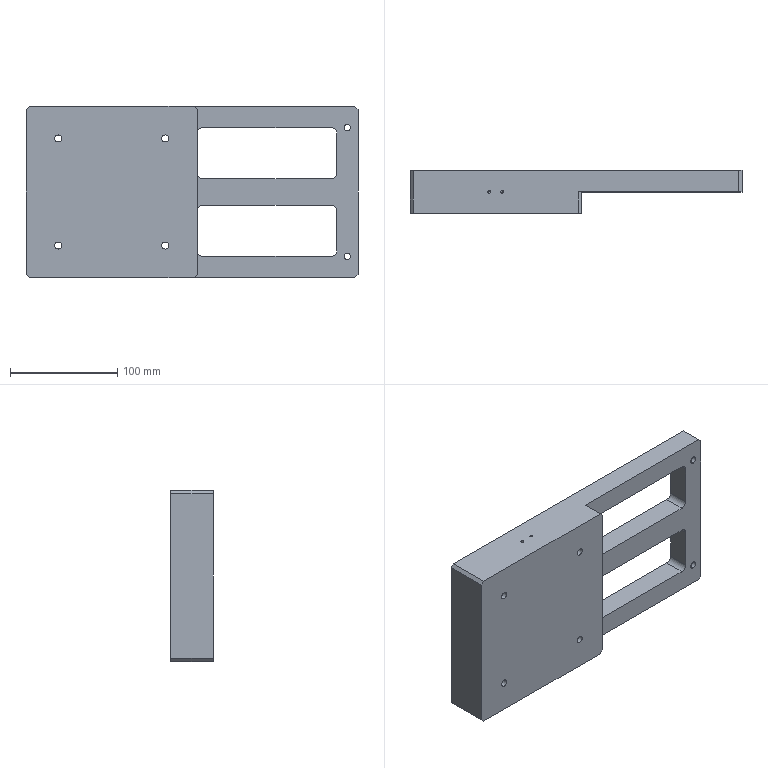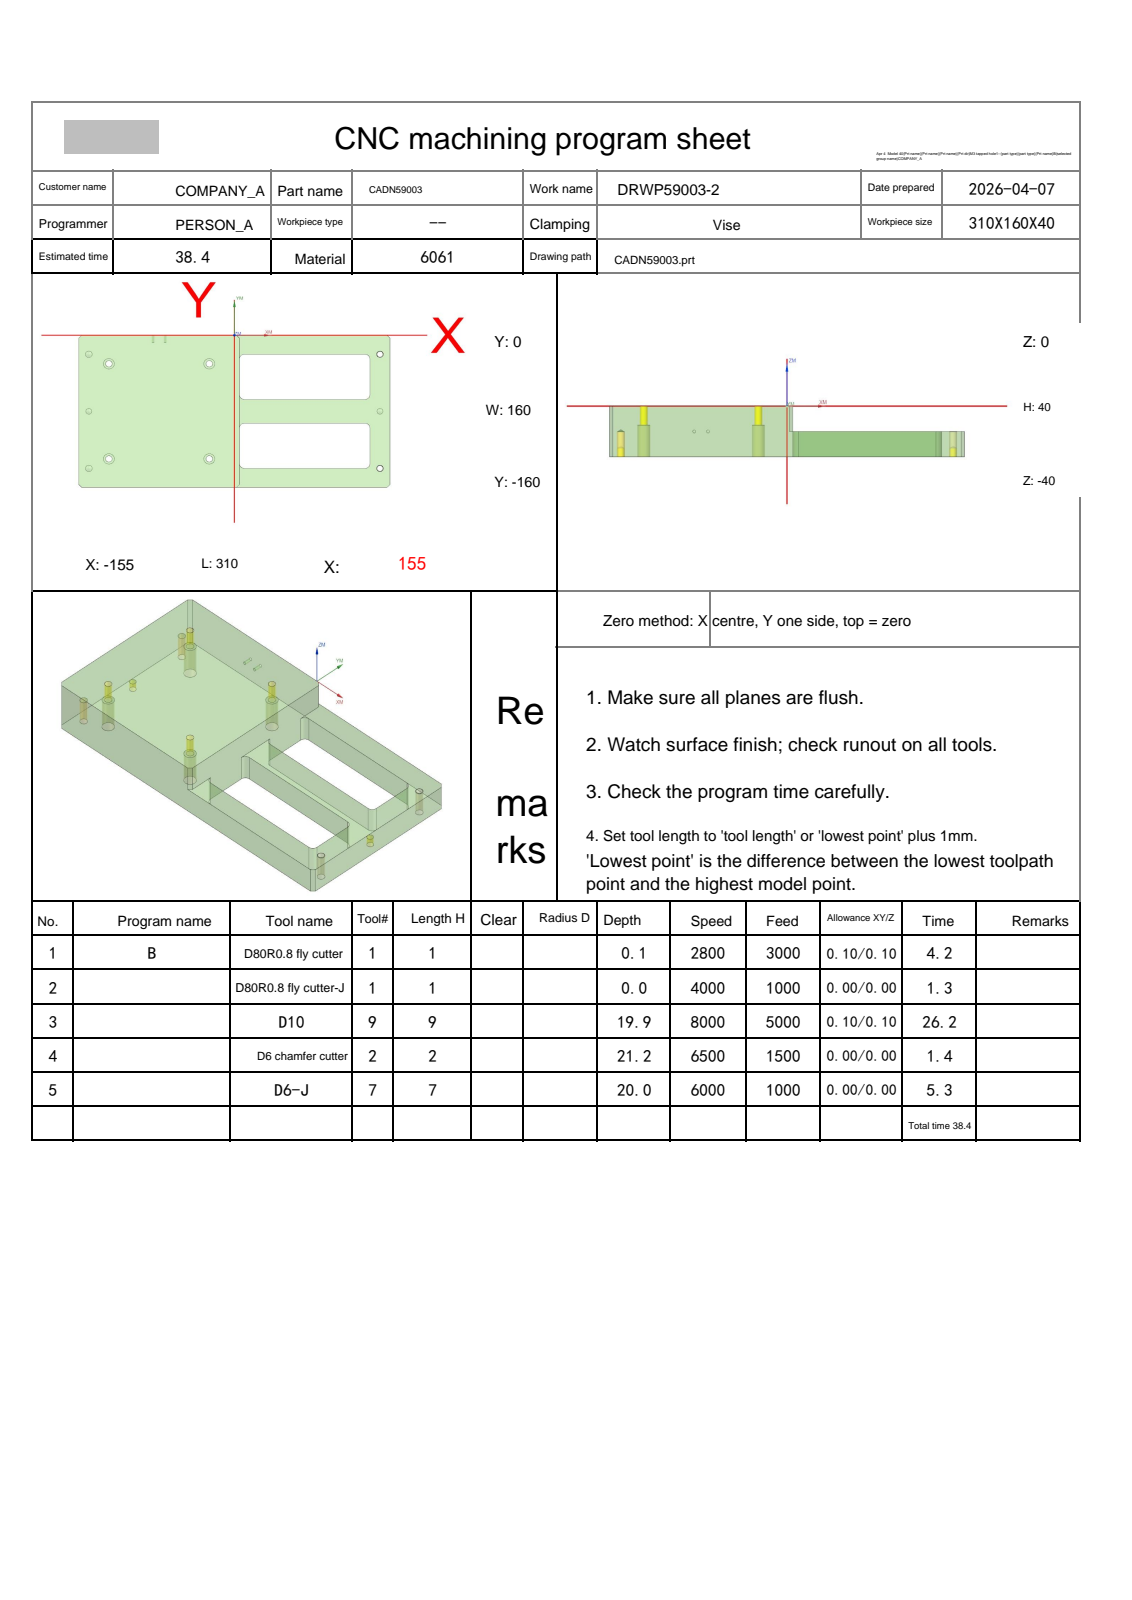NC program | NX | posted by the shop | part box 310 x 40 x 160 mm
Lines 5366 to 6465 of 6465:
N4 T02 M06
(D6 chamfer cutter  D=6. R=0. H=02 ce=0.00 di=0.00)
G00 G90 G54 X-74.614 Y-161.227 M03 S6500
G43 H02 Z20.
M08
Z.172
G01 Z-1.2 F1500.
G03 X-74.9 Y-161.027 I-1.286 J-1.532
G01 X-74.946 Y-160.997
X-75. Y-161.
X-152.
X-152.259 Y-160.966
X-152.5 Y-160.866
X-152.707 Y-160.707
X-155.707 Y-157.707
X-155.866 Y-157.5
X-155.966 Y-157.259
X-156. Y-157.
Y-3.
X-155.966 Y-2.741
X-155.866 Y-2.5
X-155.707 Y-2.293
X-152.707 Y.707
X-152.5 Y.866
X-152.259 Y.966
X-152. Y1.
X2.
X2.259 Y.966
X2.5 Y.866
X2.707 Y.707
X5.707 Y-2.293
X5.866 Y-2.5
X5.966 Y-2.741
X6. Y-3.
Y-157.
X5.966 Y-157.259
X5.866 Y-157.5
X5.707 Y-157.707
X2.707 Y-160.707
X2.5 Y-160.866
X2.259 Y-160.966
X2. Y-161.
X-75.
X-75.054 Y-160.997
X-75.1 Y-161.027
G03 X-75.386 Y-161.227 I1. J-1.732
G01 Z.172
G00 Z10.
X-24.596 Y-127.892
Z.253
G01 Z-1.2
G03 X-24.898 Y-127.718 I-1.147 J-1.638
G01 X-24.946 Y-127.692
X-25. Y-127.7
G03 X-27.3 Y-130. I0.0 J-2.3
X-25. Y-132.3 I2.3 J0.0
X-22.7 Y-130. I0.0 J2.3
X-25. Y-127.7 I-2.3 J0.0
G01 X-25.054 Y-127.692
X-25.102 Y-127.718
G03 X-25.404 Y-127.892 I.845 J-1.813
G01 Z.253
G00 Z10.
X-124.596
Z.253
G01 Z-1.2
G03 X-124.898 Y-127.718 I-1.147 J-1.638
G01 X-124.946 Y-127.692
X-125. Y-127.7
G03 X-127.3 Y-130. I0.0 J-2.3
X-125. Y-132.3 I2.3 J0.0
X-122.7 Y-130. I0.0 J2.3
X-125. Y-127.7 I-2.3 J0.0
G01 X-125.054 Y-127.692
X-125.102 Y-127.718
G03 X-125.404 Y-127.892 I.845 J-1.813
G01 Z.253
G00 Z10.
X-124.596 Y-27.892
Z.253
G01 Z-1.2
G03 X-124.898 Y-27.718 I-1.147 J-1.638
G01 X-124.946 Y-27.692
X-125. Y-27.7
G03 X-127.3 Y-30. I0.0 J-2.3
X-125. Y-32.3 I2.3 J0.0
X-122.7 Y-30. I0.0 J2.3
X-125. Y-27.7 I-2.3 J0.0
G01 X-125.054 Y-27.692
X-125.102 Y-27.718
G03 X-125.404 Y-27.892 I.845 J-1.813
G01 Z.253
G00 Z10.
X-24.596
Z.253
G01 Z-1.2
G03 X-24.898 Y-27.718 I-1.147 J-1.638
G01 X-24.946 Y-27.692
X-25. Y-27.7
G03 X-27.3 Y-30. I0.0 J-2.3
X-25. Y-32.3 I2.3 J0.0
X-22.7 Y-30. I0.0 J2.3
X-25. Y-27.7 I-2.3 J0.0
G01 X-25.054 Y-27.692
X-25.102 Y-27.718
G03 X-25.404 Y-27.892 I.845 J-1.813
G01 Z.253
G00 Z10.
X8.195 Y-65.959
Z-1.796
G01 Z-21.199
X8.217 Y-66.027
X8.262 Y-66.081
X8.269 Y-66.105
X8.293 Y-66.109
X8.469 Y-66.196
X8.965 Y-66.364
X9.478 Y-66.466
X10. Y-66.5
X130.
G03 X134. Y-62.5 I0.0 J4.
G01 Y-25.
G03 X130. Y-21. I-4. J0.0
G01 X10.
X9.478 Y-21.034
X8.965 Y-21.136
X8.469 Y-21.304
X8.293 Y-21.391
X8.271 Y-21.405
X8.249 Y-21.427
X8.206 Y-21.523
Z-1.807
G00 Z10.
X8.195 Y-138.459
Z-1.796
G01 Z-21.199
X8.217 Y-138.527
X8.262 Y-138.581
X8.269 Y-138.605
X8.293 Y-138.609
X8.469 Y-138.696
X8.965 Y-138.864
X9.478 Y-138.966
X10. Y-139.
X130.
G03 X134. Y-135. I0.0 J4.
G01 Y-97.5
G03 X130. Y-93.5 I-4. J0.0
G01 X10.
X9.478 Y-93.534
X8.965 Y-93.636
X8.469 Y-93.804
X8.293 Y-93.891
X8.271 Y-93.905
X8.249 Y-93.927
X8.206 Y-94.023
Z-1.807
G00 Z10.
X5.356 Y1.159
Z-1.793
G01 Z-21.199
G03 X5.555 Y1.019 I.9 J1.072
G01 X5.587 Y.995
X5.625 Y1.
X152.
X152.259 Y.966
X152.5 Y.866
X152.707 Y.707
X155.707 Y-2.293
X155.866 Y-2.5
X155.966 Y-2.741
X156. Y-3.
Y-157.
X155.966 Y-157.259
X155.866 Y-157.5
X155.707 Y-157.707
X152.707 Y-160.707
X152.5 Y-160.866
X152.259 Y-160.966
X152. Y-161.
X5.625
X5.587 Y-160.995
X5.555 Y-161.019
G03 X5.356 Y-161.159 I.7 J-1.212
G01 Z-1.793
G00 Z10.
X145.404 Y-18.208
Z-19.74
G01 Z-21.199
G03 X145.102 Y-18.034 I-1.147 J-1.638
G01 X145.054 Y-18.009
X145. Y-18.016
G03 X143.016 Y-20. I0.0 J-1.984
X145. Y-21.984 I1.984 J0.0
X146.984 Y-20. I0.0 J1.984
X145.345 Y-18.046 I-1.984 J0.0
G01 X145. Y-18.016
X144.946 Y-18.009
X144.898 Y-18.034
G03 X144.596 Y-18.208 I.845 J-1.813
G01 Z-19.74
G00 Z10.
X145.404 Y-138.208
Z-19.74
G01 Z-21.199
G03 X145.102 Y-138.034 I-1.147 J-1.638
G01 X145.054 Y-138.009
X145. Y-138.016
G03 X143.016 Y-140. I0.0 J-1.984
X145. Y-141.984 I1.984 J0.0
X146.984 Y-140. I0.0 J1.984
X145.345 Y-138.046 I-1.984 J0.0
G01 X145. Y-138.016
X144.946 Y-138.009
X144.898 Y-138.034
G03 X144.596 Y-138.208 I.845 J-1.813
G01 Z-19.74
G00 Z20.
G91 G28 Z0.0
M05
M09
G91 G28 Z0.0
M01
N5 T07 M06
(D6-J  D=6. R=0. H=07 ce=0.40 di=0.00)
G00 G90 G54 X158.917 Y-158.649 M03 S6000
G43 H07 Z14.5
M08
Z-18.5
G01 Z-20. F1000.
X156.6
G02 X155.4 Y-157.449 I0.0 J1.2
G01 Y-139.099
G03 X153.626 Y-116.329 I-147. J0.0
G01 X153.611 Y-116.25
X153.626 Y-116.171
G03 X155.4 Y-93.401 I-145.226 J22.77
G01 Y-66.599
G03 X153.626 Y-43.829 I-147. J0.0
G01 X153.611 Y-43.75
X153.626 Y-43.671
G03 X155.4 Y-20.901 I-145.226 J22.77
G01 Y-2.8
G03 X155.224 Y-2.376 I-.6 J0.0
G01 X152.802 Y.046
X152.633 Y.117
G03 X152.393 Y-.123 I0.0 J-.24
G01 Y-.126
G02 X152.4 Y-1.584 I-143.993 J-1.466
G01 Y-20.901
G02 X150.589 Y-43.669 I-144. J0.0
G01 X150.573 Y-43.75
X150.589 Y-43.831
G02 X152.4 Y-66.599 I-142.189 J-22.768
G01 Y-93.401
G02 X150.589 Y-116.169 I-144. J0.0
G01 X150.573 Y-116.25
X150.589 Y-116.331
G02 X152.4 Y-139.099 I-142.189 J-22.768
G01 Y-158.408
G02 X152.39 Y-160.066 I-144. J0.0
X151.851 Y-160.6 I-.54 J.006
G01 X149.93
G02 X149.39 Y-160.06 I0.0 J.54
G01 Y-160.054
G03 X149.4 Y-158.408 I-140.99 J1.646
G01 Y-139.099
G03 X147.55 Y-116.333 I-141. J0.0
G01 X147.534 Y-116.25
X147.55 Y-116.167
G03 X149.4 Y-93.401 I-139.15 J22.766
G01 Y-66.599
G03 X147.55 Y-43.833 I-141. J0.0
G01 X147.534 Y-43.75
X147.55 Y-43.667
G03 X149.4 Y-20.901 I-139.15 J22.766
G01 Y-1.584
G03 X149.391 Y.007 I-141. J-.008
X148.791 Y.6 I-.6 J-.007
G01 X146.93
G03 X146.39 Y.06 I0.0 J-.54
G01 Y.054
G02 X146.4 Y-1.584 I-137.99 J-1.646
G01 Y-20.901
G02 X144.51 Y-43.664 I-138. J0.0
G01 X144.494 Y-43.75
X144.51 Y-43.836
G02 X146.4 Y-66.599 I-136.11 J-22.763
G01 Y-93.401
G02 X144.51 Y-116.164 I-138. J0.0
G01 X144.494 Y-116.25
X144.51 Y-116.336
G02 X146.4 Y-139.099 I-136.11 J-22.763
G01 Y-158.408
G02 X146.391 Y-160.007 I-138. J0.0
X145.791 Y-160.6 I-.6 J.007
G01 X143.93
G02 X143.39 Y-160.06 I0.0 J.54
G01 Y-160.054
G03 X143.4 Y-158.408 I-134.99 J1.645
G01 Y-139.099
G03 X141.467 Y-116.338 I-135. J0.0
G01 X141.451 Y-116.25
X141.467 Y-116.162
G03 X143.4 Y-93.401 I-133.067 J22.761
G01 Y-66.599
G03 X141.467 Y-43.838 I-135. J0.0
G01 X141.451 Y-43.75
X141.467 Y-43.662
G03 X143.4 Y-20.901 I-133.067 J22.761
G01 Y-1.584
G03 X143.391 Y.007 I-135. J-.008
X142.791 Y.6 I-.6 J-.007
G01 X140.929
G03 X140.39 Y.06 I0.0 J-.54
G01 Y.054
G02 X140.4 Y-1.584 I-131.99 J-1.645
G01 Y-20.901
G02 X138.423 Y-43.659 I-132. J0.0
G01 X138.406 Y-43.75
X138.423 Y-43.841
G02 X140.4 Y-66.599 I-130.023 J-22.758
G01 Y-93.401
G02 X138.423 Y-116.159 I-132. J0.0
G01 X138.406 Y-116.25
X138.423 Y-116.341
G02 X140.4 Y-139.099 I-130.023 J-22.758
G01 Y-158.408
G02 X140.39 Y-160.007 I-132. J0.0
X139.79 Y-160.6 I-.6 J.007
G01 X137.929
G02 X137.389 Y-160.06 I0.0 J.54
G01 X137.39 Y-160.053
G03 X137.4 Y-158.408 I-128.99 J1.645
G01 Y-139.099
G03 X135.377 Y-116.343 I-129. J0.0
G01 X135.36 Y-116.25
X135.377 Y-116.157
G03 X137.4 Y-93.401 I-126.977 J22.756
G01 Y-66.599
G03 X135.377 Y-43.843 I-129. J0.0
G01 X135.36 Y-43.75
X135.377 Y-43.657
G03 X137.4 Y-20.901 I-126.977 J22.756
G01 Y-1.584
G03 X137.39 Y.007 I-129. J-.007
X136.79 Y.6 I-.6 J-.007
G01 X134.929
G03 X134.389 Y.06 I0.0 J-.54
G01 Y.053
G02 X134.4 Y-1.585 I-125.989 J-1.645
G01 Y-20.901
G02 X134.366 Y-23.839 I-126. J0.0
G01 X134.345 Y-23.895
X134.281 Y-23.903
X134.248 Y-23.853
G03 X131.76 Y-20.967 I-4.248 J-1.147
G02 X131.4 Y-20.418 I.24 J.55
G01 Y-1.585
G03 X131.39 Y.008 I-123. J-.007
X130.79 Y.6 I-.6 J-.008
G01 X128.928
G03 X128.389 Y.06 I0.0 J-.54
G01 Y.053
G02 X128.4 Y-1.585 I-119.989 J-1.645
G01 Y-20.06
G02 X127.86 Y-20.6 I-.54 J0.0
G01 X126.
G02 X125.4 Y-20. I0.0 J.6
G01 Y-1.585
G03 X125.389 Y.008 I-117. J-.007
X124.789 Y.6 I-.6 J-.008
G01 X122.928
G03 X122.388 Y.06 I0.0 J-.54
G01 Y.053
G02 X122.4 Y-1.585 I-113.988 J-1.644
G01 Y-20.06
G02 X121.86 Y-20.6 I-.54 J0.0
G01 X120.
G02 X119.4 Y-20. I0.0 J.6
G01 Y-1.585
G03 X119.388 Y.009 I-111. J-.006
X118.789 Y.6 I-.6 J-.009
G01 X116.927
G03 X116.387 Y.06 I0.0 J-.54
G01 Y.052
G02 X116.4 Y-1.586 I-107.987 J-1.644
G01 Y-20.06
G02 X115.86 Y-20.6 I-.54 J0.0
G01 X114.
G02 X113.4 Y-20. I0.0 J.6
G01 Y-1.586
G03 X113.388 Y.009 I-105. J-.006
X112.788 Y.6 I-.6 J-.009
G01 X110.926
G03 X110.387 Y.06 I0.0 J-.54
G01 Y.052
G02 X110.4 Y-1.586 I-101.987 J-1.643
G01 Y-20.06
G02 X109.86 Y-20.6 I-.54 J0.0
G01 X108.
G02 X107.4 Y-20. I0.0 J.6
G01 Y-1.586
G03 X107.387 Y.01 I-99. J-.006
X106.787 Y.6 I-.6 J-.01
G01 X104.926
G03 X104.386 Y.06 I0.0 J-.54
G01 Y.051
G02 X104.4 Y-1.586 I-95.986 J-1.643
G01 Y-20.06
G02 X103.86 Y-20.6 I-.54 J0.0
G01 X102.
G02 X101.4 Y-20. I0.0 J.6
G01 Y-1.586
G03 X101.386 Y.01 I-93. J-.005
X100.786 Y.6 I-.6 J-.01
G01 X98.925
G03 X98.385 Y.06 I0.0 J-.54
G01 Y.05
G02 X98.4 Y-1.587 I-89.985 J-1.642
G01 Y-20.06
G02 X97.86 Y-20.6 I-.54 J0.0
G01 X96.
G02 X95.4 Y-20. I0.0 J.6
G01 Y-1.587
G03 X95.385 Y.011 I-87. J-.005
X94.785 Y.6 I-.6 J-.011
G01 X92.924
G03 X92.384 Y.06 I0.0 J-.54
G01 Y.05
G02 X92.4 Y-1.587 I-83.984 J-1.641
G01 Y-20.06
G02 X91.86 Y-20.6 I-.54 J0.0
G01 X90.
G02 X89.4 Y-20. I0.0 J.6
G01 Y-1.587
G03 X89.384 Y.012 I-81. J-.005
X88.784 Y.6 I-.6 J-.012
G01 X86.922
G03 X86.383 Y.06 I0.0 J-.54
G01 Y.049
G02 X86.4 Y-1.587 I-77.983 J-1.641
G01 Y-20.06
G02 X85.86 Y-20.6 I-.54 J0.0
G01 X84.
G02 X83.4 Y-20. I0.0 J.6
G01 Y-1.587
G03 X83.383 Y.013 I-75. J-.004
X82.783 Y.6 I-.6 J-.013
G01 X80.921
G03 X80.381 Y.06 I0.0 J-.54
G01 Y.048
G02 X80.4 Y-1.588 I-71.981 J-1.64
G01 Y-20.06
G02 X79.86 Y-20.6 I-.54 J0.0
G01 X78.
G02 X77.4 Y-20. I0.0 J.6
G01 Y-1.588
G03 X77.381 Y.014 I-69. J-.004
X76.781 Y.6 I-.6 J-.014
G01 X74.919
G03 X74.379 Y.06 I0.0 J-.54
G01 X74.38 Y.047
G02 X74.4 Y-1.588 I-65.98 J-1.639
G01 Y-20.06
G02 X73.86 Y-20.6 I-.54 J0.0
G01 X72.
G02 X71.4 Y-20. I0.0 J.6
G01 Y-1.588
G03 X71.38 Y.015 I-63. J-.004
X70.78 Y.6 I-.6 J-.015
G01 X68.917
G03 X68.377 Y.06 I0.0 J-.54
G01 X68.378 Y.046
G02 X68.4 Y-1.588 I-59.978 J-1.637
G01 Y-20.06
G02 X67.86 Y-20.6 I-.54 J0.0
G01 X66.
G02 X65.4 Y-20. I0.0 J.6
G01 Y-1.588
G03 X65.377 Y.017 I-57. J-.003
X64.778 Y.6 I-.6 J-.017
G01 X62.915
G03 X62.375 Y.06 I0.0 J-.54
G01 Y.044
G02 X62.4 Y-1.589 I-53.975 J-1.636
G01 Y-20.06
G02 X61.86 Y-20.6 I-.54 J0.0
G01 X60.
G02 X59.4 Y-20. I0.0 J.6
G01 Y-1.589
G03 X59.375 Y.019 I-51. J-.003
X58.775 Y.6 I-.6 J-.019
G01 X56.912
G03 X56.372 Y.06 I0.0 J-.54
G01 Y.042
G02 X56.4 Y-1.589 I-47.972 J-1.634
G01 Y-20.06
G02 X55.86 Y-20.6 I-.54 J0.0
G01 X54.
G02 X53.4 Y-20. I0.0 J.6
G01 Y-1.589
G03 X53.371 Y.022 I-45. J-.003
X52.771 Y.6 I-.6 J-.022
G01 X50.908
G03 X50.368 Y.06 I0.0 J-.54
G01 Y.039
G02 X50.4 Y-1.589 I-41.968 J-1.631
G01 Y-20.06
G02 X49.86 Y-20.6 I-.54 J0.0
G01 X48.
G02 X47.4 Y-20. I0.0 J.6
G01 Y-1.589
G03 X47.366 Y.025 I-39. J-.002
X46.767 Y.6 I-.599 J-.025
G01 X44.902
G03 X44.363 Y.06 I0.0 J-.54
G01 Y.036
G02 X44.4 Y-1.59 I-35.963 J-1.628
G01 Y-20.06
G02 X43.86 Y-20.6 I-.54 J0.0
G01 X42.
G02 X41.4 Y-20. I0.0 J.6
G01 Y-1.59
G03 X41.36 Y.029 I-33. J-.002
X40.761 Y.6 I-.599 J-.029
G01 X38.895
G03 X38.355 Y.06 I0.0 J-.54
G01 X38.356 Y.031
G02 X38.4 Y-1.59 I-29.956 J-1.623
G01 Y-20.06
G02 X37.86 Y-20.6 I-.54 J0.0
G01 X36.
G02 X35.4 Y-20. I0.0 J.6
G01 Y-1.59
G03 X35.351 Y.036 I-27. J-.002
X34.752 Y.6 I-.599 J-.036
G01 X32.884
G03 X32.344 Y.06 I0.0 J-.54
G01 X32.346 Y.024
G02 X32.4 Y-1.59 I-23.946 J-1.616
G01 Y-20.06
G02 X31.86 Y-20.6 I-.54 J0.0
G01 X30.
G02 X29.4 Y-20. I0.0 J.6
G01 Y-1.59
G03 X29.336 Y.047 I-21. J-.001
X28.738 Y.6 I-.598 J-.047
G01 X26.866
G03 X26.326 Y.06 I0.0 J-.54
G01 X26.328 Y.012
G02 X26.4 Y-1.591 I-17.928 J-1.604
G01 Y-20.06
G02 X25.86 Y-20.6 I-.54 J0.0
G01 X24.
G02 X23.4 Y-20. I0.0 J.6
G01 Y-1.591
G03 X23.308 Y.066 I-15. J-.001
X22.712 Y.6 I-.596 J-.066
G01 X20.762
G03 X20.282 Y.12 I0.0 J-.48
G01 X20.287 Y.054
G02 X20.4 Y-1.592 I-11.887 J-1.646
G01 Y-20.06
G02 X19.86 Y-20.6 I-.54 J0.0
G01 X18.
G02 X17.4 Y-20. I0.0 J.6
G01 Y-1.592
G03 X17.237 Y.114 I-9. J0.0
X16.648 Y.6 I-.589 J-.114
G01 X14.57
G03 X14.151 Y.18 I0.0 J-.42
G01 X14.167 Y.064
G02 X14.4 Y-1.592 I-5.767 J-1.656
G01 Y-20.06
G02 X13.86 Y-20.6 I-.54 J0.0
G01 X12.
G02 X11.4 Y-20. I0.0 J.6
G01 Y-1.592
G03 X10.572 Y.478 I-3. J0.0
X10.296 Y.642 I-.434 J-.414
G01 X6.791 Y1.603
X6.633 Y1.624
G03 X6.033 Y1.024 I0.0 J-.6
X6.208 Y.6 I.6 J0.0
G01 X8.4 Y-1.592
Y-20.901
G03 X9.6 Y-22.101 I1.2 J0.0
G01 X9.891 Y-24.208
Z-18.5
G00 X130.8 Y-61.911
G01 Z-20.
X135.519
G03 X134.352 Y-63.111 I.033 J-1.2
G01 X134.353 Y-63.144
G02 X134.4 Y-66.599 I-125.953 J-3.455
G01 Y-93.401
G02 X134.366 Y-96.339 I-126. J0.0
G01 X134.345 Y-96.395
X134.281 Y-96.403
X134.248 Y-96.353
G03 X131.76 Y-93.467 I-4.248 J-1.147
G02 X131.4 Y-92.918 I.24 J.55
G01 Y-67.219
G03 X130.98 Y-66.799 I-.42 J0.0
G01 X130.895 Y-66.808
G02 X130. Y-66.9 I-.895 J4.308
G01 X129.
G03 X128.4 Y-67.5 I0.0 J-.6
G01 Y-92.56
G02 X127.86 Y-93.1 I-.54 J0.0
G01 X126.
G02 X125.4 Y-92.5 I0.0 J.6
G01 Y-67.44
G03 X124.86 Y-66.9 I-.54 J0.0
G01 X123.
G03 X122.4 Y-67.5 I0.0 J-.6
G01 Y-92.56
G02 X121.86 Y-93.1 I-.54 J0.0
G01 X120.
G02 X119.4 Y-92.5 I0.0 J.6
G01 Y-67.44
G03 X118.86 Y-66.9 I-.54 J0.0
G01 X117.
G03 X116.4 Y-67.5 I0.0 J-.6
G01 Y-92.56
G02 X115.86 Y-93.1 I-.54 J0.0
G01 X114.
G02 X113.4 Y-92.5 I0.0 J.6
G01 Y-67.44
G03 X112.86 Y-66.9 I-.54 J0.0
G01 X111.
G03 X110.4 Y-67.5 I0.0 J-.6
G01 Y-92.56
G02 X109.86 Y-93.1 I-.54 J0.0
G01 X108.
G02 X107.4 Y-92.5 I0.0 J.6
G01 Y-67.44
G03 X106.86 Y-66.9 I-.54 J0.0
G01 X105.
G03 X104.4 Y-67.5 I0.0 J-.6
G01 Y-92.56
G02 X103.86 Y-93.1 I-.54 J0.0
G01 X102.
G02 X101.4 Y-92.5 I0.0 J.6
G01 Y-67.44
G03 X100.86 Y-66.9 I-.54 J0.0
G01 X99.
G03 X98.4 Y-67.5 I0.0 J-.6
G01 Y-92.56
G02 X97.86 Y-93.1 I-.54 J0.0
G01 X96.
G02 X95.4 Y-92.5 I0.0 J.6
G01 Y-67.44
G03 X94.86 Y-66.9 I-.54 J0.0
G01 X93.
G03 X92.4 Y-67.5 I0.0 J-.6
G01 Y-92.56
G02 X91.86 Y-93.1 I-.54 J0.0
G01 X90.
G02 X89.4 Y-92.5 I0.0 J.6
G01 Y-67.44
G03 X88.86 Y-66.9 I-.54 J0.0
G01 X87.
G03 X86.4 Y-67.5 I0.0 J-.6
G01 Y-92.56
G02 X85.86 Y-93.1 I-.54 J0.0
G01 X84.
G02 X83.4 Y-92.5 I0.0 J.6
G01 Y-67.44
G03 X82.86 Y-66.9 I-.54 J0.0
G01 X81.
G03 X80.4 Y-67.5 I0.0 J-.6
G01 Y-92.56
G02 X79.86 Y-93.1 I-.54 J0.0
G01 X78.
G02 X77.4 Y-92.5 I0.0 J.6
G01 Y-67.44
G03 X76.86 Y-66.9 I-.54 J0.0
G01 X75.
G03 X74.4 Y-67.5 I0.0 J-.6
G01 Y-92.56
G02 X73.86 Y-93.1 I-.54 J0.0
G01 X72.
G02 X71.4 Y-92.5 I0.0 J.6
G01 Y-67.44
G03 X70.86 Y-66.9 I-.54 J0.0
G01 X69.
G03 X68.4 Y-67.5 I0.0 J-.6
G01 Y-92.56
G02 X67.86 Y-93.1 I-.54 J0.0
G01 X66.
G02 X65.4 Y-92.5 I0.0 J.6
G01 Y-67.44
G03 X64.86 Y-66.9 I-.54 J0.0
G01 X62.94
G03 X62.4 Y-67.44 I0.0 J-.54
G01 Y-92.56
G02 X61.86 Y-93.1 I-.54 J0.0
G01 X60.
G02 X59.4 Y-92.5 I0.0 J.6
G01 Y-67.44
G03 X58.86 Y-66.9 I-.54 J0.0
G01 X57.
G03 X56.4 Y-67.5 I0.0 J-.6
G01 Y-92.56
G02 X55.86 Y-93.1 I-.54 J0.0
G01 X54.
G02 X53.4 Y-92.5 I0.0 J.6
G01 Y-67.44
G03 X52.86 Y-66.9 I-.54 J0.0
G01 X51.
G03 X50.4 Y-67.5 I0.0 J-.6
G01 Y-92.56
G02 X49.86 Y-93.1 I-.54 J0.0
G01 X48.
G02 X47.4 Y-92.5 I0.0 J.6
G01 Y-67.44
G03 X46.86 Y-66.9 I-.54 J0.0
G01 X44.94
G03 X44.4 Y-67.44 I0.0 J-.54
G01 Y-92.56
G02 X43.86 Y-93.1 I-.54 J0.0
G01 X42.
G02 X41.4 Y-92.5 I0.0 J.6
G01 Y-67.44
G03 X40.86 Y-66.9 I-.54 J0.0
G01 X39.
G03 X38.4 Y-67.5 I0.0 J-.6
G01 Y-92.56
G02 X37.86 Y-93.1 I-.54 J0.0
G01 X36.
G02 X35.4 Y-92.5 I0.0 J.6
G01 Y-67.44
G03 X34.86 Y-66.9 I-.54 J0.0
G01 X33.
G03 X32.4 Y-67.5 I0.0 J-.6
G01 Y-92.56
G02 X31.86 Y-93.1 I-.54 J0.0
G01 X30.
G02 X29.4 Y-92.5 I0.0 J.6
G01 Y-67.44
G03 X28.86 Y-66.9 I-.54 J0.0
G01 X27.
G03 X26.4 Y-67.5 I0.0 J-.6
G01 Y-92.56
G02 X25.86 Y-93.1 I-.54 J0.0
G01 X24.
G02 X23.4 Y-92.5 I0.0 J.6
G01 Y-67.44
G03 X22.86 Y-66.9 I-.54 J0.0
G01 X21.
G03 X20.4 Y-67.5 I0.0 J-.6
G01 Y-92.56
G02 X19.86 Y-93.1 I-.54 J0.0
G01 X18.
G02 X17.4 Y-92.5 I0.0 J.6
G01 Y-67.44
G03 X16.86 Y-66.9 I-.54 J0.0
G01 X15.
G03 X14.4 Y-67.5 I0.0 J-.6
G01 Y-92.56
G02 X13.86 Y-93.1 I-.54 J0.0
G01 X12.
G02 X11.4 Y-92.5 I0.0 J.6
G01 Y-67.5
G03 X10.8 Y-66.9 I-.6 J0.0
G01 X10.
G02 X9.487 Y-66.252 I2.677 J2.648
G01 X9.436 Y-66.187
G03 X9. Y-65.999 I-.436 J-.412
X8.4 Y-66.599 I0.0 J-.6
G01 Y-93.401
G03 X9.6 Y-94.601 I1.2 J0.0
G01 X9.891 Y-96.708
Z-18.5
G00 X130.8 Y-134.411
G01 Z-20.
X135.519
G03 X134.352 Y-135.611 I.033 J-1.2
G01 X134.353 Y-135.644
G02 X134.4 Y-139.099 I-125.953 J-3.455
G01 Y-158.408
G02 X134.39 Y-160.008 I-126. J0.0
X133.79 Y-160.6 I-.6 J.008
G01 X131.929
G02 X131.389 Y-160.06 I0.0 J.54
G01 Y-160.053
G03 X131.4 Y-158.408 I-122.989 J1.645
G01 Y-139.719
G03 X130.98 Y-139.299 I-.42 J0.0
G01 X130.895 Y-139.308
G02 X130. Y-139.4 I-.895 J4.308
G01 X129.
G03 X128.4 Y-140. I0.0 J-.6
G01 Y-158.408
G02 X128.389 Y-160.008 I-120. J0.0
X127.789 Y-160.6 I-.6 J.008
G01 X125.928
G02 X125.388 Y-160.06 I0.0 J.54
G01 Y-160.053
G03 X125.4 Y-158.408 I-116.988 J1.644
G01 Y-139.94
G03 X124.86 Y-139.4 I-.54 J0.0
G01 X123.
G03 X122.4 Y-140. I0.0 J-.6
G01 Y-158.408
G02 X122.389 Y-160.008 I-114. J0.0
X121.789 Y-160.6 I-.6 J.008
G01 X119.927
G02 X119.388 Y-160.06 I0.0 J.54
G01 Y-160.052
G03 X119.4 Y-158.408 I-110.988 J1.644
G01 Y-139.94
G03 X118.86 Y-139.4 I-.54 J0.0
G01 X117.
G03 X116.4 Y-140. I0.0 J-.6
G01 Y-158.408
G02 X116.388 Y-160.009 I-108. J0.0
X115.788 Y-160.6 I-.6 J.009
G01 X113.927
G02 X113.387 Y-160.06 I0.0 J.54
G01 Y-160.052
G03 X113.4 Y-158.408 I-104.987 J1.644
G01 Y-139.94
G03 X112.86 Y-139.4 I-.54 J0.0
G01 X111.
G03 X110.4 Y-140. I0.0 J-.6
G01 Y-158.408
G02 X110.387 Y-160.009 I-102. J0.0
X109.788 Y-160.6 I-.6 J.009
G01 X107.926
G02 X107.386 Y-160.06 I0.0 J.54
G01 Y-160.051
G03 X107.4 Y-158.408 I-98.986 J1.643
G01 Y-139.94
G03 X106.86 Y-139.4 I-.54 J0.0
G01 X105.
G03 X104.4 Y-140. I0.0 J-.6
G01 Y-158.408
G02 X104.387 Y-160.01 I-96. J0.0
X103.787 Y-160.6 I-.6 J.01
G01 X101.925
G02 X101.385 Y-160.06 I0.0 J.54
G01 Y-160.051
G03 X101.4 Y-158.408 I-92.985 J1.642
G01 Y-139.94
G03 X100.86 Y-139.4 I-.54 J0.0
G01 X99.
G03 X98.4 Y-140. I0.0 J-.6
G01 Y-158.408
G02 X98.386 Y-160.011 I-90. J0.0
X97.786 Y-160.6 I-.6 J.011
G01 X95.924
G02 X95.384 Y-160.06 I0.0 J.54
G01 X95.385 Y-160.05
G03 X95.4 Y-158.408 I-86.985 J1.642
G01 Y-139.94
G03 X94.86 Y-139.4 I-.54 J0.0
G01 X93.
G03 X92.4 Y-140. I0.0 J-.6
G01 Y-158.408
G02 X92.385 Y-160.011 I-84. J0.0
X91.785 Y-160.6 I-.6 J.011
G01 X89.923
G02 X89.383 Y-160.06 I0.0 J.54
G01 Y-160.049
G03 X89.4 Y-158.408 I-80.983 J1.641
G01 Y-139.94
G03 X88.86 Y-139.4 I-.54 J0.0
G01 X87.
G03 X86.4 Y-140. I0.0 J-.6
G01 Y-158.408
G02 X86.384 Y-160.012 I-78. J0.0
X85.784 Y-160.6 I-.6 J.012
G01 X83.922
G02 X83.382 Y-160.06 I0.0 J.54
G01 Y-160.049
G03 X83.4 Y-158.408 I-74.982 J1.64
G01 Y-139.94
G03 X82.86 Y-139.4 I-.54 J0.0
G01 X81.
G03 X80.4 Y-140. I0.0 J-.6
G01 Y-158.408
G02 X80.382 Y-160.013 I-72. J0.0
X79.782 Y-160.6 I-.6 J.013
G01 X77.92
G02 X77.38 Y-160.06 I0.0 J.54
G01 X77.381 Y-160.047
G03 X77.4 Y-158.408 I-68.981 J1.639
G01 Y-139.94
G03 X76.86 Y-139.4 I-.54 J0.0
G01 X75.
G03 X74.4 Y-140. I0.0 J-.6
G01 Y-158.408
G02 X74.38 Y-160.015 I-66. J0.0
X73.781 Y-160.6 I-.6 J.015
G01 X71.918
G02 X71.379 Y-160.06 I0.0 J.54
G01 Y-160.046
G03 X71.4 Y-158.408 I-62.979 J1.638
G01 Y-139.94
G03 X70.86 Y-139.4 I-.54 J0.0
G01 X69.
G03 X68.4 Y-140. I0.0 J-.6
G01 Y-158.408
G02 X68.378 Y-160.016 I-60. J0.0
X67.779 Y-160.6 I-.6 J.016
G01 X65.916
G02 X65.376 Y-160.06 I0.0 J.54
G01 X65.377 Y-160.045
G03 X65.4 Y-158.408 I-56.977 J1.636
G01 Y-139.94
G03 X64.86 Y-139.4 I-.54 J0.0
G01 X63.
G03 X62.4 Y-140. I0.0 J-.6
G01 Y-158.408
G02 X62.376 Y-160.018 I-54. J0.0
X61.776 Y-160.6 I-.6 J.018
G01 X59.913
G02 X59.374 Y-160.06 I0.0 J.54
G01 Y-160.043
G03 X59.4 Y-158.408 I-50.974 J1.635
G01 Y-139.94
G03 X58.86 Y-139.4 I-.54 J0.0
G01 X57.
G03 X56.4 Y-140. I0.0 J-.6
G01 Y-158.408
G02 X56.373 Y-160.02 I-48. J0.0
X55.773 Y-160.6 I-.6 J.02
G01 X53.91
G02 X53.37 Y-160.06 I0.0 J.54
G01 Y-160.041
G03 X53.4 Y-158.408 I-44.97 J1.632
G01 Y-139.94
G03 X52.86 Y-139.4 I-.54 J0.0
G01 X51.
G03 X50.4 Y-140. I0.0 J-.6
G01 Y-158.408
G02 X50.369 Y-160.023 I-42. J0.0
X49.769 Y-160.6 I-.6 J.023
G01 X47.905
G02 X47.365 Y-160.06 I0.0 J.54
G01 X47.366 Y-160.038
G03 X47.4 Y-158.408 I-38.966 J1.629
G01 Y-139.94
G03 X46.86 Y-139.4 I-.54 J0.0
G01 X45.
G03 X44.4 Y-140. I0.0 J-.6
G01 Y-158.408
G02 X44.364 Y-160.027 I-36. J0.0
X43.764 Y-160.6 I-.599 J.027
G01 X41.899
G02 X41.359 Y-160.06 I0.0 J.54
G01 X41.36 Y-160.034
G03 X41.4 Y-158.408 I-32.96 J1.625
G01 Y-139.94
G03 X40.86 Y-139.4 I-.54 J0.0
G01 X39.
G03 X38.4 Y-140. I0.0 J-.6
G01 Y-158.408
G02 X38.356 Y-160.032 I-30. J0.0
X37.757 Y-160.6 I-.599 J.032
G01 X35.89
G02 X35.35 Y-160.06 I0.0 J.54
G01 X35.351 Y-160.028
G03 X35.4 Y-158.408 I-26.951 J1.62
G01 Y-139.94
G03 X34.86 Y-139.4 I-.54 J0.0
G01 X33.
G03 X32.4 Y-140. I0.0 J-.6
G01 Y-158.408
G02 X32.344 Y-160.041 I-24. J0.0
X31.746 Y-160.6 I-.599 J.041
G01 X29.876
G02 X29.337 Y-160.06 I0.0 J.54
G01 X29.338 Y-160.019
G03 X29.4 Y-158.408 I-20.938 J1.611
G01 Y-139.94
G03 X28.86 Y-139.4 I-.54 J0.0
G01 X27.
G03 X26.4 Y-140. I0.0 J-.6
G01 Y-158.408
G02 X26.325 Y-160.055 I-18. J0.0
X25.727 Y-160.6 I-.597 J.055
G01 X23.785
G02 X23.305 Y-160.12 I0.0 J.48
G01 X23.308 Y-160.067
G03 X23.4 Y-158.408 I-14.908 J1.659
G01 Y-139.94
G03 X22.86 Y-139.4 I-.54 J0.0
G01 X21.
G03 X20.4 Y-140. I0.0 J-.6
G01 Y-158.408
G02 X20.282 Y-160.084 I-12. J0.0
X19.688 Y-160.6 I-.594 J.084
G01 X17.724
G02 X17.244 Y-160.12 I0.0 J.48
G01 X17.252 Y-160.034
G03 X17.4 Y-158.408 I-8.852 J1.625
G01 Y-139.94
G03 X16.86 Y-139.4 I-.54 J0.0
G01 X15.
G03 X14.4 Y-140. I0.0 J-.6
G01 Y-158.408
G02 X14.133 Y-160.177 I-6. J0.0
X13.56 Y-160.6 I-.573 J.177
G01 X10.986
G02 X10.746 Y-160.36 I0.0 J.24
G01 X10.795 Y-160.216
G03 X11.4 Y-158.408 I-2.395 J1.807
G01 Y-140.
G03 X10.8 Y-139.4 I-.6 J0.0
G01 X10.
G02 X9.487 Y-138.752 I2.677 J2.648
G01 X9.436 Y-138.687
G03 X9. Y-138.499 I-.436 J-.412
X8.4 Y-139.099 I0.0 J-.6
G01 Y-158.408
X6.208 Y-160.6
G03 X5.857 Y-161.449 I.849 J-.849
X6.208 Y-162.297 I1.2 J0.0
G01 X8.111 Y-164.2
Z-18.5
G00 Z14.5
G00 G90 X4.176 Y3.473 M03 S6000
Z9.5
Z-4.
G01 Z-5. F1000.
G41 D07
X4.052 Y3.316
G03 X3.858 Y2.758 I.706 J-.559
X4.121 Y2.121 I.9 J0.0
G01 X7.121 Y-.879
G02 X8. Y-3. I-2.121 J-2.121
G01 Y-157.
G02 X7.121 Y-159.121 I-3. J0.0
G01 X4.121 Y-162.121
G03 X3.858 Y-162.758 I.636 J-.636
X4.052 Y-163.316 I.9 J0.0
G01 G40 X4.176 Y-163.473
Z-4.
G00 Z9.5
Y3.473
Z-9.
G01 Z-10.
G41 D07
X4.052 Y3.316
G03 X3.858 Y2.758 I.706 J-.559
X4.121 Y2.121 I.9 J0.0
G01 X7.121 Y-.879
G02 X8. Y-3. I-2.121 J-2.121
G01 Y-157.
G02 X7.121 Y-159.121 I-3. J0.0
G01 X4.121 Y-162.121
G03 X3.858 Y-162.758 I.636 J-.636
X4.052 Y-163.316 I.9 J0.0
G01 G40 X4.176 Y-163.473
Z-9.
G00 Z9.5
Y3.473
Z-14.
G01 Z-15.
G41 D07
X4.052 Y3.316
G03 X3.858 Y2.758 I.706 J-.559
X4.121 Y2.121 I.9 J0.0
G01 X7.121 Y-.879
G02 X8. Y-3. I-2.121 J-2.121
G01 Y-157.
G02 X7.121 Y-159.121 I-3. J0.0
G01 X4.121 Y-162.121
G03 X3.858 Y-162.758 I.636 J-.636
X4.052 Y-163.316 I.9 J0.0
G01 G40 X4.176 Y-163.473
Z-14.
G00 Z9.5
Y3.473
Z-19.
G01 Z-20.
G41 D07
X4.052 Y3.316
G03 X3.858 Y2.758 I.706 J-.559
X4.121 Y2.121 I.9 J0.0
G01 X7.121 Y-.879
G02 X8. Y-3. I-2.121 J-2.121
G01 Y-157.
G02 X7.121 Y-159.121 I-3. J0.0
G01 X4.121 Y-162.121
G03 X3.858 Y-162.758 I.636 J-.636
X4.052 Y-163.316 I.9 J0.0
G01 G40 X4.176 Y-163.473
Z-19.
G00 Z9.5
M05
M09
G91 G28 Z0.0
G91 G28 Y0.0
M30
%